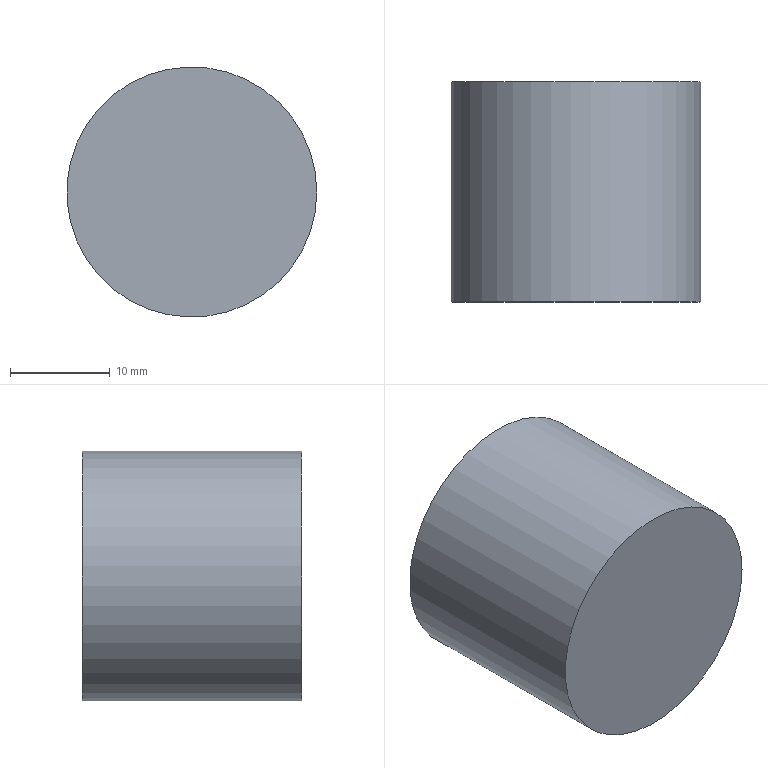Part | NX | features solid 2 | 1 solid | 3 faces | box 25 x 22 x 25 mm | volume 10799 mm3 | plane 2 | cylinder 1 | commonest cylinder face diameters 25 x1
STEP:
#1=CARTESIAN_POINT('',(542.5,750.001,130.));
#2=VERTEX_POINT('',#1);
#3=CARTESIAN_POINT('',(530.,750.001,130.));
#4=DIRECTION('',(0.,1.,0.));
#5=DIRECTION('',(1.,0.,0.));
#6=AXIS2_PLACEMENT_3D('',#3,#4,#5);
#7=CIRCLE('',#6,12.5);
#8=EDGE_CURVE('',#2,#2,#7,.T.);
#9=ORIENTED_EDGE('',*,*,#8,.F.);
#10=EDGE_LOOP('',(#9));
#11=FACE_BOUND('',#10,.T.);
#12=CARTESIAN_POINT('',(542.5,728.001,130.));
#13=VERTEX_POINT('',#12);
#14=CARTESIAN_POINT('',(530.,728.001,130.));
#15=DIRECTION('',(0.,1.,0.));
#16=DIRECTION('',(1.,0.,0.));
#17=AXIS2_PLACEMENT_3D('',#14,#15,#16);
#18=CIRCLE('',#17,12.5);
#19=EDGE_CURVE('',#13,#13,#18,.T.);
#20=ORIENTED_EDGE('',*,*,#19,.T.);
#21=EDGE_LOOP('',(#20));
#22=FACE_BOUND('',#21,.T.);
#23=CARTESIAN_POINT('',(530.,750.001,130.));
#24=DIRECTION('',(0.,-1.,0.));
#25=DIRECTION('',(-1.,0.,0.));
#26=AXIS2_PLACEMENT_3D('',#23,#24,#25);
#27=CYLINDRICAL_SURFACE('',#26,12.5);
#28=ADVANCED_FACE('',(#11,#22),#27,.T.);
#29=ORIENTED_EDGE('',*,*,#8,.T.);
#30=EDGE_LOOP('',(#29));
#31=FACE_BOUND('',#30,.T.);
#32=CARTESIAN_POINT('',(530.,750.001,130.));
#33=DIRECTION('',(0.,1.,0.));
#34=DIRECTION('',(1.,0.,0.));
#35=AXIS2_PLACEMENT_3D('',#32,#33,#34);
#36=PLANE('',#35);
#37=ADVANCED_FACE('',(#31),#36,.T.);
#38=ORIENTED_EDGE('',*,*,#19,.F.);
#39=EDGE_LOOP('',(#38));
#40=FACE_BOUND('',#39,.T.);
#41=CARTESIAN_POINT('',(530.,728.001,130.));
#42=DIRECTION('',(0.,1.,0.));
#43=DIRECTION('',(1.,0.,0.));
#44=AXIS2_PLACEMENT_3D('',#41,#42,#43);
#45=PLANE('',#44);
#46=ADVANCED_FACE('',(#40),#45,.F.);
#47=CLOSED_SHELL('',(#28,#37,#46));
#48=MANIFOLD_SOLID_BREP('',#47);
#49=(LENGTH_UNIT()NAMED_UNIT(*)SI_UNIT(.MILLI.,.METRE.));
#50=UNCERTAINTY_MEASURE_WITH_UNIT(LENGTH_MEASURE(0.00001),#49,'','');
#51=(NAMED_UNIT(*)PLANE_ANGLE_UNIT()SI_UNIT($,.RADIAN.));
#52=(NAMED_UNIT(*)SI_UNIT($,.STERADIAN.)SOLID_ANGLE_UNIT());
#53=(GEOMETRIC_REPRESENTATION_CONTEXT(3)GLOBAL_UNCERTAINTY_ASSIGNED_CONTEXT((#50))GLOBAL_UNIT_ASSIGNED_CONTEXT((#49,#51,#52))REPRESENTATION_CONTEXT('',''));
#54=ADVANCED_BREP_SHAPE_REPRESENTATION('',(#48),#53);